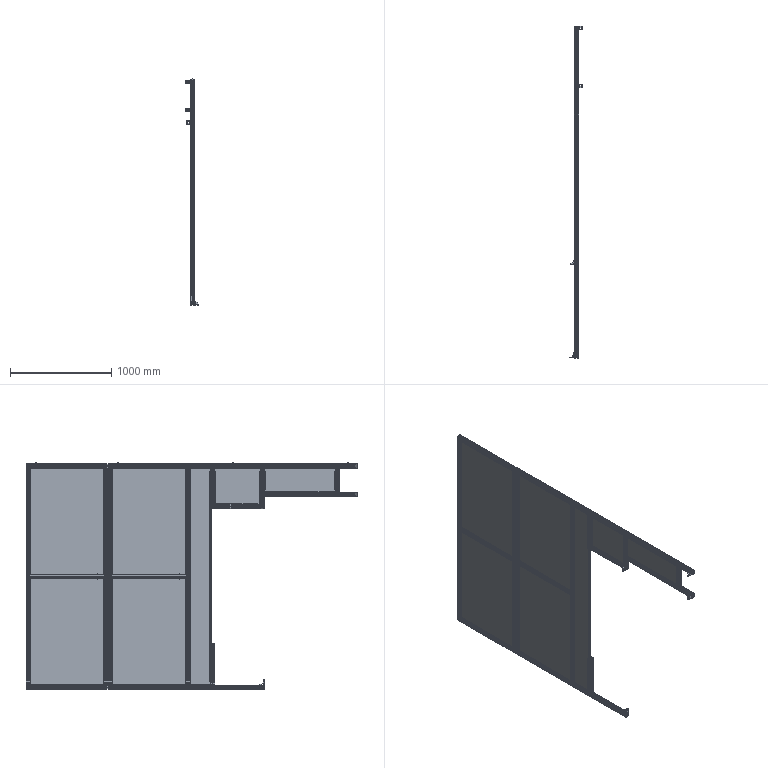Part | SolidWorks | features ReferencePattern 104, MirrorCompFeat 10, LocalLPattern 4, DerivedHolePattern 1 | 109 solids | 6191 faces | volume 29193097 mm3 | plane 4441 | cylinder 1566 | cone 184 | commonest cylinder face diameters 2 x231 6.8 x206 1 x161 19 x132 0.8 x84 5 x64